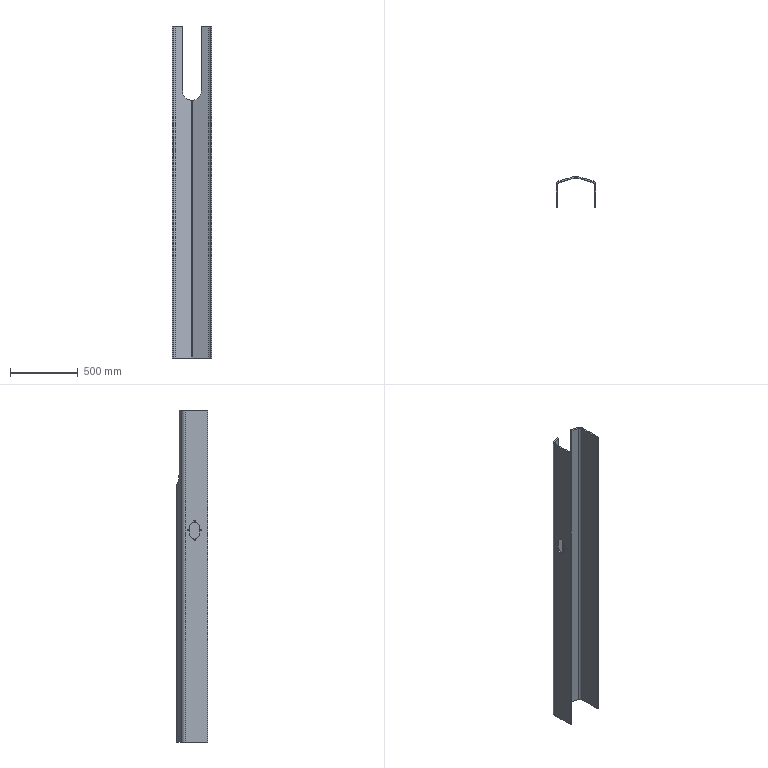Part | SolidWorks | features ICE 2, Extrusion 1, HoleWzd 1 | 1 solid | 36 faces | box 295 x 232 x 2455 mm | volume 15250128 mm3 | cylinder 19 | plane 17 | commonest cylinder face diameters 8.5 x8 40 x3 60 x3 80 x3 140 x2
STEP:
#1=CARTESIAN_POINT('',(-137.5,147.,1560.75));
#2=VERTEX_POINT('',#1);
#3=CARTESIAN_POINT('',(-137.5,147.,1569.25));
#4=VERTEX_POINT('',#3);
#5=CARTESIAN_POINT('',(-137.5,147.,1565.));
#6=DIRECTION('',(-1.,0.,0.));
#7=DIRECTION('',(0.,0.,1.));
#8=AXIS2_PLACEMENT_3D('',#5,#6,#7);
#9=CIRCLE('',#8,4.25);
#10=EDGE_CURVE('',#2,#4,#9,.T.);
#11=ORIENTED_EDGE('',*,*,#10,.F.);
#12=CARTESIAN_POINT('',(-147.5,147.,1560.75));
#13=VERTEX_POINT('',#12);
#14=CARTESIAN_POINT('',(-147.5,147.,1560.75));
#15=DIRECTION('',(-1.,0.,0.));
#16=VECTOR('',#15,1000.);
#17=LINE('',#14,#16);
#18=EDGE_CURVE('',#2,#13,#17,.T.);
#19=ORIENTED_EDGE('',*,*,#18,.T.);
#20=CARTESIAN_POINT('',(-147.5,147.,1569.25));
#21=VERTEX_POINT('',#20);
#22=CARTESIAN_POINT('',(-147.5,147.,1565.));
#23=DIRECTION('',(-1.,0.,0.));
#24=DIRECTION('',(0.,0.,1.));
#25=AXIS2_PLACEMENT_3D('',#22,#23,#24);
#26=CIRCLE('',#25,4.25);
#27=EDGE_CURVE('',#13,#21,#26,.T.);
#28=ORIENTED_EDGE('',*,*,#27,.T.);
#29=CARTESIAN_POINT('',(-147.5,147.,1569.25));
#30=DIRECTION('',(-1.,0.,0.));
#31=VECTOR('',#30,1000.);
#32=LINE('',#29,#31);
#33=EDGE_CURVE('',#4,#21,#32,.T.);
#34=ORIENTED_EDGE('',*,*,#33,.F.);
#35=EDGE_LOOP('',(#11,#19,#28,#34));
#36=FACE_OUTER_BOUND('',#35,.T.);
#37=CARTESIAN_POINT('',(-147.5,147.,1565.));
#38=DIRECTION('',(-1.,0.,0.));
#39=DIRECTION('',(0.,0.,1.));
#40=AXIS2_PLACEMENT_3D('',#37,#38,#39);
#41=CYLINDRICAL_SURFACE('',#40,4.25);
#42=ADVANCED_FACE('',(#36),#41,.F.);
#43=CARTESIAN_POINT('',(-137.5,47.,1560.75));
#44=VERTEX_POINT('',#43);
#45=CARTESIAN_POINT('',(-137.5,47.,1569.25));
#46=VERTEX_POINT('',#45);
#47=CARTESIAN_POINT('',(-137.5,47.,1565.));
#48=DIRECTION('',(-1.,0.,0.));
#49=DIRECTION('',(0.,0.,1.));
#50=AXIS2_PLACEMENT_3D('',#47,#48,#49);
#51=CIRCLE('',#50,4.25);
#52=EDGE_CURVE('',#44,#46,#51,.T.);
#53=ORIENTED_EDGE('',*,*,#52,.F.);
#54=CARTESIAN_POINT('',(-147.5,47.,1560.75));
#55=VERTEX_POINT('',#54);
#56=CARTESIAN_POINT('',(-147.5,47.,1560.75));
#57=DIRECTION('',(-1.,0.,0.));
#58=VECTOR('',#57,1000.);
#59=LINE('',#56,#58);
#60=EDGE_CURVE('',#44,#55,#59,.T.);
#61=ORIENTED_EDGE('',*,*,#60,.T.);
#62=CARTESIAN_POINT('',(-147.5,47.,1569.25));
#63=VERTEX_POINT('',#62);
#64=CARTESIAN_POINT('',(-147.5,47.,1565.));
#65=DIRECTION('',(-1.,0.,0.));
#66=DIRECTION('',(0.,0.,1.));
#67=AXIS2_PLACEMENT_3D('',#64,#65,#66);
#68=CIRCLE('',#67,4.25);
#69=EDGE_CURVE('',#55,#63,#68,.T.);
#70=ORIENTED_EDGE('',*,*,#69,.T.);
#71=CARTESIAN_POINT('',(-147.5,47.,1569.25));
#72=DIRECTION('',(-1.,0.,0.));
#73=VECTOR('',#72,1000.);
#74=LINE('',#71,#73);
#75=EDGE_CURVE('',#46,#63,#74,.T.);
#76=ORIENTED_EDGE('',*,*,#75,.F.);
#77=EDGE_LOOP('',(#53,#61,#70,#76));
#78=FACE_OUTER_BOUND('',#77,.T.);
#79=CARTESIAN_POINT('',(-147.5,47.,1565.));
#80=DIRECTION('',(-1.,0.,0.));
#81=DIRECTION('',(0.,0.,1.));
#82=AXIS2_PLACEMENT_3D('',#79,#80,#81);
#83=CYLINDRICAL_SURFACE('',#82,4.25);
#84=ADVANCED_FACE('',(#78),#83,.F.);
#85=CARTESIAN_POINT('',(-137.5,97.,1490.75));
#86=VERTEX_POINT('',#85);
#87=CARTESIAN_POINT('',(-137.5,97.,1499.25));
#88=VERTEX_POINT('',#87);
#89=CARTESIAN_POINT('',(-137.5,97.,1495.));
#90=DIRECTION('',(-1.,0.,0.));
#91=DIRECTION('',(0.,0.,1.));
#92=AXIS2_PLACEMENT_3D('',#89,#90,#91);
#93=CIRCLE('',#92,4.25);
#94=EDGE_CURVE('',#86,#88,#93,.T.);
#95=ORIENTED_EDGE('',*,*,#94,.F.);
#96=CARTESIAN_POINT('',(-147.5,97.,1490.75));
#97=VERTEX_POINT('',#96);
#98=CARTESIAN_POINT('',(-147.5,97.,1490.75));
#99=DIRECTION('',(-1.,0.,0.));
#100=VECTOR('',#99,1000.);
#101=LINE('',#98,#100);
#102=EDGE_CURVE('',#86,#97,#101,.T.);
#103=ORIENTED_EDGE('',*,*,#102,.T.);
#104=CARTESIAN_POINT('',(-147.5,97.,1499.25));
#105=VERTEX_POINT('',#104);
#106=CARTESIAN_POINT('',(-147.5,97.,1495.));
#107=DIRECTION('',(-1.,0.,0.));
#108=DIRECTION('',(0.,0.,1.));
#109=AXIS2_PLACEMENT_3D('',#106,#107,#108);
#110=CIRCLE('',#109,4.25);
#111=EDGE_CURVE('',#97,#105,#110,.T.);
#112=ORIENTED_EDGE('',*,*,#111,.T.);
#113=CARTESIAN_POINT('',(-147.5,97.,1499.25));
#114=DIRECTION('',(-1.,0.,0.));
#115=VECTOR('',#114,1000.);
#116=LINE('',#113,#115);
#117=EDGE_CURVE('',#88,#105,#116,.T.);
#118=ORIENTED_EDGE('',*,*,#117,.F.);
#119=EDGE_LOOP('',(#95,#103,#112,#118));
#120=FACE_OUTER_BOUND('',#119,.T.);
#121=CARTESIAN_POINT('',(-147.5,97.,1495.));
#122=DIRECTION('',(-1.,0.,0.));
#123=DIRECTION('',(0.,0.,1.));
#124=AXIS2_PLACEMENT_3D('',#121,#122,#123);
#125=CYLINDRICAL_SURFACE('',#124,4.25);
#126=ADVANCED_FACE('',(#120),#125,.F.);
#127=CARTESIAN_POINT('',(-137.5,97.,1630.75));
#128=VERTEX_POINT('',#127);
#129=CARTESIAN_POINT('',(-137.5,97.,1639.25));
#130=VERTEX_POINT('',#129);
#131=CARTESIAN_POINT('',(-137.5,97.,1635.));
#132=DIRECTION('',(-1.,0.,0.));
#133=DIRECTION('',(0.,0.,1.));
#134=AXIS2_PLACEMENT_3D('',#131,#132,#133);
#135=CIRCLE('',#134,4.25);
#136=EDGE_CURVE('',#128,#130,#135,.T.);
#137=ORIENTED_EDGE('',*,*,#136,.F.);
#138=CARTESIAN_POINT('',(-147.5,97.,1630.75));
#139=VERTEX_POINT('',#138);
#140=CARTESIAN_POINT('',(-147.5,97.,1630.75));
#141=DIRECTION('',(-1.,0.,0.));
#142=VECTOR('',#141,1000.);
#143=LINE('',#140,#142);
#144=EDGE_CURVE('',#128,#139,#143,.T.);
#145=ORIENTED_EDGE('',*,*,#144,.T.);
#146=CARTESIAN_POINT('',(-147.5,97.,1639.25));
#147=VERTEX_POINT('',#146);
#148=CARTESIAN_POINT('',(-147.5,97.,1635.));
#149=DIRECTION('',(-1.,0.,0.));
#150=DIRECTION('',(0.,0.,1.));
#151=AXIS2_PLACEMENT_3D('',#148,#149,#150);
#152=CIRCLE('',#151,4.25);
#153=EDGE_CURVE('',#139,#147,#152,.T.);
#154=ORIENTED_EDGE('',*,*,#153,.T.);
#155=CARTESIAN_POINT('',(-147.5,97.,1639.25));
#156=DIRECTION('',(-1.,0.,0.));
#157=VECTOR('',#156,1000.);
#158=LINE('',#155,#157);
#159=EDGE_CURVE('',#130,#147,#158,.T.);
#160=ORIENTED_EDGE('',*,*,#159,.F.);
#161=EDGE_LOOP('',(#137,#145,#154,#160));
#162=FACE_OUTER_BOUND('',#161,.T.);
#163=CARTESIAN_POINT('',(-147.5,97.,1635.));
#164=DIRECTION('',(-1.,0.,0.));
#165=DIRECTION('',(0.,0.,1.));
#166=AXIS2_PLACEMENT_3D('',#163,#164,#165);
#167=CYLINDRICAL_SURFACE('',#166,4.25);
#168=ADVANCED_FACE('',(#162),#167,.F.);
#169=CARTESIAN_POINT('',(-137.5,97.,1625.));
#170=VERTEX_POINT('',#169);
#171=CARTESIAN_POINT('',(-137.5,137.,1585.));
#172=VERTEX_POINT('',#171);
#173=CARTESIAN_POINT('',(-137.5,97.,1585.));
#174=DIRECTION('',(-1.,0.,0.));
#175=DIRECTION('',(0.,0.,1.));
#176=AXIS2_PLACEMENT_3D('',#173,#174,#175);
#177=CIRCLE('',#176,40.);
#178=EDGE_CURVE('',#170,#172,#177,.T.);
#179=ORIENTED_EDGE('',*,*,#178,.F.);
#180=CARTESIAN_POINT('',(-147.5,97.,1625.));
#181=VERTEX_POINT('',#180);
#182=CARTESIAN_POINT('',(-137.5,97.,1625.));
#183=DIRECTION('',(-1.,0.,0.));
#184=VECTOR('',#183,1000.);
#185=LINE('',#182,#184);
#186=EDGE_CURVE('',#170,#181,#185,.T.);
#187=ORIENTED_EDGE('',*,*,#186,.T.);
#188=CARTESIAN_POINT('',(-147.5,137.,1585.));
#189=VERTEX_POINT('',#188);
#190=CARTESIAN_POINT('',(-147.5,97.,1585.));
#191=DIRECTION('',(-1.,0.,0.));
#192=DIRECTION('',(0.,0.,1.));
#193=AXIS2_PLACEMENT_3D('',#190,#191,#192);
#194=CIRCLE('',#193,40.);
#195=EDGE_CURVE('',#181,#189,#194,.T.);
#196=ORIENTED_EDGE('',*,*,#195,.T.);
#197=CARTESIAN_POINT('',(-137.5,137.,1585.));
#198=DIRECTION('',(-1.,0.,0.));
#199=VECTOR('',#198,1000.);
#200=LINE('',#197,#199);
#201=EDGE_CURVE('',#172,#189,#200,.T.);
#202=ORIENTED_EDGE('',*,*,#201,.F.);
#203=EDGE_LOOP('',(#179,#187,#196,#202));
#204=FACE_OUTER_BOUND('',#203,.T.);
#205=CARTESIAN_POINT('',(-137.5,97.,1585.));
#206=DIRECTION('',(-1.,0.,0.));
#207=DIRECTION('',(0.,0.,1.));
#208=AXIS2_PLACEMENT_3D('',#205,#206,#207);
#209=CYLINDRICAL_SURFACE('',#208,40.);
#210=ADVANCED_FACE('',(#204),#209,.F.);
#211=CARTESIAN_POINT('',(8.771,230.689,1905.552));
#212=VERTEX_POINT('',#211);
#213=CARTESIAN_POINT('',(0.,232.,1905.));
#214=VERTEX_POINT('',#213);
#215=CARTESIAN_POINT('',(8.771,230.689,1905.552));
#216=CARTESIAN_POINT('',(7.345,231.125,1905.372));
#217=CARTESIAN_POINT('',(5.901,231.451,1905.234));
#218=CARTESIAN_POINT('',(2.978,231.888,1905.048));
#219=CARTESIAN_POINT('',(1.498,232.,1905.));
#220=CARTESIAN_POINT('',(0.,232.,1905.));
#221=B_SPLINE_CURVE_WITH_KNOTS('',3,(#215,#216,#217,#218,#219,#220),.UNSPECIFIED.,.F.,.F.,(4,2,4),(0.,0.004443,0.008885),.UNSPECIFIED.);
#222=EDGE_CURVE('',#212,#214,#221,.T.);
#223=ORIENTED_EDGE('',*,*,#222,.T.);
#224=CARTESIAN_POINT('',(0.,222.,1905.));
#225=VERTEX_POINT('',#224);
#226=CARTESIAN_POINT('',(0.,232.,1905.));
#227=DIRECTION('',(0.,-1.,0.));
#228=VECTOR('',#227,1000.);
#229=LINE('',#226,#228);
#230=EDGE_CURVE('',#214,#225,#229,.T.);
#231=ORIENTED_EDGE('',*,*,#230,.T.);
#232=CARTESIAN_POINT('',(5.847,221.126,1905.245));
#233=VERTEX_POINT('',#232);
#234=CARTESIAN_POINT('',(0.,222.,1905.));
#235=CARTESIAN_POINT('',(0.4958,222.,1905.));
#236=CARTESIAN_POINT('',(0.9948,221.981,1905.005));
#237=CARTESIAN_POINT('',(1.983,221.908,1905.026));
#238=CARTESIAN_POINT('',(2.473,221.853,1905.042));
#239=CARTESIAN_POINT('',(3.936,221.634,1905.104));
#240=CARTESIAN_POINT('',(4.898,221.416,1905.165));
#241=CARTESIAN_POINT('',(5.847,221.126,1905.245));
#242=B_SPLINE_CURVE_WITH_KNOTS('',3,(#234,#235,#236,#237,#238,#239,#240,#241),.UNSPECIFIED.,.F.,.F.,(4,2,2,4),(0.005917,0.00739,0.008863,0.01181),.UNSPECIFIED.);
#243=EDGE_CURVE('',#225,#233,#242,.T.);
#244=ORIENTED_EDGE('',*,*,#243,.T.);
#245=CARTESIAN_POINT('',(70.,201.513,1975.));
#246=VERTEX_POINT('',#245);
#247=CARTESIAN_POINT('',(5.847,221.126,1905.245));
#248=CARTESIAN_POINT('',(44.049,209.447,1908.447));
#249=CARTESIAN_POINT('',(70.,201.513,1936.664));
#250=CARTESIAN_POINT('',(70.,201.513,1975.));
#251=(BOUNDED_CURVE()B_SPLINE_CURVE(3,(#247,#248,#249,#250),.UNSPECIFIED.,.F.,.T.)B_SPLINE_CURVE_WITH_KNOTS((4,4),(4.796,6.283),.UNSPECIFIED.)CURVE()GEOMETRIC_REPRESENTATION_ITEM()RATIONAL_B_SPLINE_CURVE((1.,0.824,0.824,1.))REPRESENTATION_ITEM(''));
#252=EDGE_CURVE('',#233,#246,#251,.T.);
#253=ORIENTED_EDGE('',*,*,#252,.T.);
#254=CARTESIAN_POINT('',(70.,211.97,1975.));
#255=VERTEX_POINT('',#254);
#256=CARTESIAN_POINT('',(70.,232.,1975.));
#257=DIRECTION('',(0.,-1.,0.));
#258=VECTOR('',#257,1000.);
#259=LINE('',#256,#258);
#260=EDGE_CURVE('',#255,#246,#259,.T.);
#261=ORIENTED_EDGE('',*,*,#260,.F.);
#262=CARTESIAN_POINT('',(70.,211.97,1975.));
#263=CARTESIAN_POINT('',(70.,211.97,1937.969));
#264=CARTESIAN_POINT('',(45.51,219.457,1910.192));
#265=CARTESIAN_POINT('',(8.771,230.689,1905.552));
#266=(BOUNDED_CURVE()B_SPLINE_CURVE(3,(#262,#263,#264,#265),.UNSPECIFIED.,.F.,.T.)B_SPLINE_CURVE_WITH_KNOTS((4,4),(0.,1.445),.UNSPECIFIED.)CURVE()GEOMETRIC_REPRESENTATION_ITEM()RATIONAL_B_SPLINE_CURVE((1.,0.8334,0.8334,1.))REPRESENTATION_ITEM(''));
#267=EDGE_CURVE('',#255,#212,#266,.T.);
#268=ORIENTED_EDGE('',*,*,#267,.T.);
#269=EDGE_LOOP('',(#223,#231,#244,#253,#261,#268));
#270=FACE_OUTER_BOUND('',#269,.T.);
#271=CARTESIAN_POINT('',(0.,232.,1975.));
#272=DIRECTION('',(0.,-1.,0.));
#273=DIRECTION('',(0.,0.,-1.));
#274=AXIS2_PLACEMENT_3D('',#271,#272,#273);
#275=CYLINDRICAL_SURFACE('',#274,70.);
#276=ADVANCED_FACE('',(#270),#275,.F.);
#277=CARTESIAN_POINT('',(-70.,201.513,1975.));
#278=VERTEX_POINT('',#277);
#279=CARTESIAN_POINT('',(-5.847,221.126,1905.245));
#280=VERTEX_POINT('',#279);
#281=CARTESIAN_POINT('',(-70.,201.513,1975.));
#282=CARTESIAN_POINT('',(-70.,201.513,1936.664));
#283=CARTESIAN_POINT('',(-44.049,209.447,1908.447));
#284=CARTESIAN_POINT('',(-5.847,221.126,1905.245));
#285=(BOUNDED_CURVE()B_SPLINE_CURVE(3,(#281,#282,#283,#284),.UNSPECIFIED.,.F.,.T.)B_SPLINE_CURVE_WITH_KNOTS((4,4),(0.,1.487),.UNSPECIFIED.)CURVE()GEOMETRIC_REPRESENTATION_ITEM()RATIONAL_B_SPLINE_CURVE((1.,0.824,0.824,1.))REPRESENTATION_ITEM(''));
#286=EDGE_CURVE('',#278,#280,#285,.T.);
#287=ORIENTED_EDGE('',*,*,#286,.F.);
#288=CARTESIAN_POINT('',(-70.,201.513,2455.));
#289=VERTEX_POINT('',#288);
#290=CARTESIAN_POINT('',(-70.,201.513,2455.));
#291=DIRECTION('',(0.,0.,-1.));
#292=VECTOR('',#291,1000.);
#293=LINE('',#290,#292);
#294=EDGE_CURVE('',#289,#278,#293,.T.);
#295=ORIENTED_EDGE('',*,*,#294,.F.);
#296=CARTESIAN_POINT('',(-123.347,185.203,2455.));
#297=VERTEX_POINT('',#296);
#298=CARTESIAN_POINT('',(-123.347,185.203,2455.));
#299=DIRECTION('',(0.9563,0.2924,0.));
#300=VECTOR('',#299,1000.);
#301=LINE('',#298,#300);
#302=EDGE_CURVE('',#297,#289,#301,.T.);
#303=ORIENTED_EDGE('',*,*,#302,.F.);
#304=CARTESIAN_POINT('',(-123.347,185.203,0.));
#305=VERTEX_POINT('',#304);
#306=CARTESIAN_POINT('',(-123.347,185.203,2455.));
#307=DIRECTION('',(0.,0.,-1.));
#308=VECTOR('',#307,1000.);
#309=LINE('',#306,#308);
#310=EDGE_CURVE('',#297,#305,#309,.T.);
#311=ORIENTED_EDGE('',*,*,#310,.T.);
#312=CARTESIAN_POINT('',(-5.847,221.126,0.));
#313=VERTEX_POINT('',#312);
#314=CARTESIAN_POINT('',(-123.347,185.203,0.));
#315=DIRECTION('',(0.9563,0.2924,0.));
#316=VECTOR('',#315,1000.);
#317=LINE('',#314,#316);
#318=EDGE_CURVE('',#305,#313,#317,.T.);
#319=ORIENTED_EDGE('',*,*,#318,.T.);
#320=CARTESIAN_POINT('',(-5.847,221.126,2455.));
#321=DIRECTION('',(0.,0.,-1.));
#322=VECTOR('',#321,1000.);
#323=LINE('',#320,#322);
#324=EDGE_CURVE('',#280,#313,#323,.T.);
#325=ORIENTED_EDGE('',*,*,#324,.F.);
#326=EDGE_LOOP('',(#287,#295,#303,#311,#319,#325));
#327=FACE_OUTER_BOUND('',#326,.T.);
#328=CARTESIAN_POINT('',(-123.347,185.203,2455.));
#329=DIRECTION('',(-0.2924,0.9563,0.));
#330=DIRECTION('',(-0.9563,-0.2924,0.));
#331=AXIS2_PLACEMENT_3D('',#328,#329,#330);
#332=PLANE('',#331);
#333=ADVANCED_FACE('',(#327),#332,.F.);
#334=CARTESIAN_POINT('',(-5.847,221.126,1905.245));
#335=CARTESIAN_POINT('',(-4.894,221.418,1905.165));
#336=CARTESIAN_POINT('',(-3.93,221.635,1905.104));
#337=CARTESIAN_POINT('',(-1.981,221.926,1905.021));
#338=CARTESIAN_POINT('',(-0.9957,222.,1905.));
#339=CARTESIAN_POINT('',(0.,222.,1905.));
#340=B_SPLINE_CURVE_WITH_KNOTS('',3,(#334,#335,#336,#337,#338,#339),.UNSPECIFIED.,.F.,.F.,(4,2,4),(0.,0.002958,0.005917),.UNSPECIFIED.);
#341=EDGE_CURVE('',#280,#225,#340,.T.);
#342=ORIENTED_EDGE('',*,*,#341,.F.);
#343=ORIENTED_EDGE('',*,*,#324,.T.);
#344=CARTESIAN_POINT('',(5.847,221.126,0.));
#345=VERTEX_POINT('',#344);
#346=CARTESIAN_POINT('',(0.,202.,0.));
#347=DIRECTION('',(0.,0.,-1.));
#348=DIRECTION('',(1.,0.,0.));
#349=AXIS2_PLACEMENT_3D('',#346,#347,#348);
#350=CIRCLE('',#349,20.);
#351=EDGE_CURVE('',#313,#345,#350,.T.);
#352=ORIENTED_EDGE('',*,*,#351,.T.);
#353=CARTESIAN_POINT('',(5.847,221.126,2455.));
#354=DIRECTION('',(0.,0.,-1.));
#355=VECTOR('',#354,1000.);
#356=LINE('',#353,#355);
#357=EDGE_CURVE('',#233,#345,#356,.T.);
#358=ORIENTED_EDGE('',*,*,#357,.F.);
#359=ORIENTED_EDGE('',*,*,#243,.F.);
#360=EDGE_LOOP('',(#342,#343,#352,#358,#359));
#361=FACE_OUTER_BOUND('',#360,.T.);
#362=CARTESIAN_POINT('',(0.,202.,2455.));
#363=DIRECTION('',(0.,0.,-1.));
#364=DIRECTION('',(-1.,0.,0.));
#365=AXIS2_PLACEMENT_3D('',#362,#363,#364);
#366=CYLINDRICAL_SURFACE('',#365,20.);
#367=ADVANCED_FACE('',(#361),#366,.F.);
#368=ORIENTED_EDGE('',*,*,#252,.F.);
#369=ORIENTED_EDGE('',*,*,#357,.T.);
#370=CARTESIAN_POINT('',(123.347,185.203,0.));
#371=VERTEX_POINT('',#370);
#372=CARTESIAN_POINT('',(123.347,185.203,0.));
#373=DIRECTION('',(0.9563,-0.2924,0.));
#374=VECTOR('',#373,1000.);
#375=LINE('',#372,#374);
#376=EDGE_CURVE('',#345,#371,#375,.T.);
#377=ORIENTED_EDGE('',*,*,#376,.T.);
#378=CARTESIAN_POINT('',(123.347,185.203,2455.));
#379=VERTEX_POINT('',#378);
#380=CARTESIAN_POINT('',(123.347,185.203,2455.));
#381=DIRECTION('',(0.,0.,-1.));
#382=VECTOR('',#381,1000.);
#383=LINE('',#380,#382);
#384=EDGE_CURVE('',#379,#371,#383,.T.);
#385=ORIENTED_EDGE('',*,*,#384,.F.);
#386=CARTESIAN_POINT('',(70.,201.513,2455.));
#387=VERTEX_POINT('',#386);
#388=CARTESIAN_POINT('',(123.347,185.203,2455.));
#389=DIRECTION('',(0.9563,-0.2924,0.));
#390=VECTOR('',#389,1000.);
#391=LINE('',#388,#390);
#392=EDGE_CURVE('',#387,#379,#391,.T.);
#393=ORIENTED_EDGE('',*,*,#392,.F.);
#394=CARTESIAN_POINT('',(70.,201.513,2455.));
#395=DIRECTION('',(0.,0.,1.));
#396=VECTOR('',#395,1000.);
#397=LINE('',#394,#396);
#398=EDGE_CURVE('',#246,#387,#397,.T.);
#399=ORIENTED_EDGE('',*,*,#398,.F.);
#400=EDGE_LOOP('',(#368,#369,#377,#385,#393,#399));
#401=FACE_OUTER_BOUND('',#400,.T.);
#402=CARTESIAN_POINT('',(123.347,185.203,2455.));
#403=DIRECTION('',(0.2924,0.9563,0.));
#404=DIRECTION('',(-0.9563,0.2924,0.));
#405=AXIS2_PLACEMENT_3D('',#402,#403,#404);
#406=PLANE('',#405);
#407=ADVANCED_FACE('',(#401),#406,.F.);
#408=ORIENTED_EDGE('',*,*,#267,.F.);
#409=CARTESIAN_POINT('',(70.,211.97,2455.));
#410=VERTEX_POINT('',#409);
#411=CARTESIAN_POINT('',(70.,211.97,2455.));
#412=DIRECTION('',(0.,0.,-1.));
#413=VECTOR('',#412,1000.);
#414=LINE('',#411,#413);
#415=EDGE_CURVE('',#410,#255,#414,.T.);
#416=ORIENTED_EDGE('',*,*,#415,.F.);
#417=CARTESIAN_POINT('',(126.271,194.766,2455.));
#418=VERTEX_POINT('',#417);
#419=CARTESIAN_POINT('',(126.271,194.766,2455.));
#420=DIRECTION('',(-0.9563,0.2924,0.));
#421=VECTOR('',#420,1000.);
#422=LINE('',#419,#421);
#423=EDGE_CURVE('',#418,#410,#422,.T.);
#424=ORIENTED_EDGE('',*,*,#423,.F.);
#425=CARTESIAN_POINT('',(126.271,194.766,0.));
#426=VERTEX_POINT('',#425);
#427=CARTESIAN_POINT('',(126.271,194.766,2455.));
#428=DIRECTION('',(0.,0.,-1.));
#429=VECTOR('',#428,1000.);
#430=LINE('',#427,#429);
#431=EDGE_CURVE('',#418,#426,#430,.T.);
#432=ORIENTED_EDGE('',*,*,#431,.T.);
#433=CARTESIAN_POINT('',(8.771,230.689,0.));
#434=VERTEX_POINT('',#433);
#435=CARTESIAN_POINT('',(126.271,194.766,0.));
#436=DIRECTION('',(-0.9563,0.2924,0.));
#437=VECTOR('',#436,1000.);
#438=LINE('',#435,#437);
#439=EDGE_CURVE('',#426,#434,#438,.T.);
#440=ORIENTED_EDGE('',*,*,#439,.T.);
#441=CARTESIAN_POINT('',(8.771,230.689,2455.));
#442=DIRECTION('',(0.,0.,-1.));
#443=VECTOR('',#442,1000.);
#444=LINE('',#441,#443);
#445=EDGE_CURVE('',#212,#434,#444,.T.);
#446=ORIENTED_EDGE('',*,*,#445,.F.);
#447=EDGE_LOOP('',(#408,#416,#424,#432,#440,#446));
#448=FACE_OUTER_BOUND('',#447,.T.);
#449=CARTESIAN_POINT('',(126.271,194.766,2455.));
#450=DIRECTION('',(-0.2924,-0.9563,0.));
#451=DIRECTION('',(0.9563,-0.2924,0.));
#452=AXIS2_PLACEMENT_3D('',#449,#450,#451);
#453=PLANE('',#452);
#454=ADVANCED_FACE('',(#448),#453,.F.);
#455=ORIENTED_EDGE('',*,*,#222,.F.);
#456=ORIENTED_EDGE('',*,*,#445,.T.);
#457=CARTESIAN_POINT('',(-8.771,230.689,0.));
#458=VERTEX_POINT('',#457);
#459=CARTESIAN_POINT('',(0.,202.,0.));
#460=DIRECTION('',(0.,0.,1.));
#461=DIRECTION('',(1.,0.,0.));
#462=AXIS2_PLACEMENT_3D('',#459,#460,#461);
#463=CIRCLE('',#462,30.);
#464=EDGE_CURVE('',#434,#458,#463,.T.);
#465=ORIENTED_EDGE('',*,*,#464,.T.);
#466=CARTESIAN_POINT('',(-8.771,230.689,1905.552));
#467=VERTEX_POINT('',#466);
#468=CARTESIAN_POINT('',(-8.771,230.689,2455.));
#469=DIRECTION('',(0.,0.,-1.));
#470=VECTOR('',#469,1000.);
#471=LINE('',#468,#470);
#472=EDGE_CURVE('',#467,#458,#471,.T.);
#473=ORIENTED_EDGE('',*,*,#472,.F.);
#474=CARTESIAN_POINT('',(0.,232.,1905.));
#475=CARTESIAN_POINT('',(-0.747,232.,1905.));
#476=CARTESIAN_POINT('',(-1.496,231.972,1905.012));
#477=CARTESIAN_POINT('',(-2.978,231.861,1905.059));
#478=CARTESIAN_POINT('',(-3.714,231.778,1905.095));
#479=CARTESIAN_POINT('',(-5.907,231.45,1905.234));
#480=CARTESIAN_POINT('',(-7.349,231.124,1905.372));
#481=CARTESIAN_POINT('',(-8.771,230.689,1905.552));
#482=B_SPLINE_CURVE_WITH_KNOTS('',3,(#474,#475,#476,#477,#478,#479,#480,#481),.UNSPECIFIED.,.F.,.F.,(4,2,2,4),(0.008885,0.0111,0.01332,0.01775),.UNSPECIFIED.);
#483=EDGE_CURVE('',#214,#467,#482,.T.);
#484=ORIENTED_EDGE('',*,*,#483,.F.);
#485=EDGE_LOOP('',(#455,#456,#465,#473,#484));
#486=FACE_OUTER_BOUND('',#485,.T.);
#487=CARTESIAN_POINT('',(0.,202.,2455.));
#488=DIRECTION('',(0.,0.,-1.));
#489=DIRECTION('',(-1.,0.,0.));
#490=AXIS2_PLACEMENT_3D('',#487,#488,#489);
#491=CYLINDRICAL_SURFACE('',#490,30.);
#492=ADVANCED_FACE('',(#486),#491,.T.);
#493=CARTESIAN_POINT('',(-70.,211.97,1975.));
#494=VERTEX_POINT('',#493);
#495=CARTESIAN_POINT('',(-8.771,230.689,1905.552));
#496=CARTESIAN_POINT('',(-45.51,219.457,1910.192));
#497=CARTESIAN_POINT('',(-70.,211.97,1937.969));
#498=CARTESIAN_POINT('',(-70.,211.97,1975.));
#499=(BOUNDED_CURVE()B_SPLINE_CURVE(3,(#495,#496,#497,#498),.UNSPECIFIED.,.F.,.F.)B_SPLINE_CURVE_WITH_KNOTS((4,4),(4.838,6.283),.UNSPECIFIED.)CURVE()GEOMETRIC_REPRESENTATION_ITEM()RATIONAL_B_SPLINE_CURVE((1.,0.8334,0.8334,1.))REPRESENTATION_ITEM(''));
#500=EDGE_CURVE('',#467,#494,#499,.T.);
#501=ORIENTED_EDGE('',*,*,#500,.F.);
#502=ORIENTED_EDGE('',*,*,#472,.T.);
#503=CARTESIAN_POINT('',(-126.271,194.766,0.));
#504=VERTEX_POINT('',#503);
#505=CARTESIAN_POINT('',(-126.271,194.766,0.));
#506=DIRECTION('',(-0.9563,-0.2924,0.));
#507=VECTOR('',#506,1000.);
#508=LINE('',#505,#507);
#509=EDGE_CURVE('',#458,#504,#508,.T.);
#510=ORIENTED_EDGE('',*,*,#509,.T.);
#511=CARTESIAN_POINT('',(-126.271,194.766,2455.));
#512=VERTEX_POINT('',#511);
#513=CARTESIAN_POINT('',(-126.271,194.766,2455.));
#514=DIRECTION('',(0.,0.,-1.));
#515=VECTOR('',#514,1000.);
#516=LINE('',#513,#515);
#517=EDGE_CURVE('',#512,#504,#516,.T.);
#518=ORIENTED_EDGE('',*,*,#517,.F.);
#519=CARTESIAN_POINT('',(-70.,211.97,2455.));
#520=VERTEX_POINT('',#519);
#521=CARTESIAN_POINT('',(-126.271,194.766,2455.));
#522=DIRECTION('',(-0.9563,-0.2924,0.));
#523=VECTOR('',#522,1000.);
#524=LINE('',#521,#523);
#525=EDGE_CURVE('',#520,#512,#524,.T.);
#526=ORIENTED_EDGE('',*,*,#525,.F.);
#527=CARTESIAN_POINT('',(-70.,211.97,2455.));
#528=DIRECTION('',(0.,0.,1.));
#529=VECTOR('',#528,1000.);
#530=LINE('',#527,#529);
#531=EDGE_CURVE('',#494,#520,#530,.T.);
#532=ORIENTED_EDGE('',*,*,#531,.F.);
#533=EDGE_LOOP('',(#501,#502,#510,#518,#526,#532));
#534=FACE_OUTER_BOUND('',#533,.T.);
#535=CARTESIAN_POINT('',(-126.271,194.766,2455.));
#536=DIRECTION('',(0.2924,-0.9563,0.));
#537=DIRECTION('',(0.9563,0.2924,0.));
#538=AXIS2_PLACEMENT_3D('',#535,#536,#537);
#539=PLANE('',#538);
#540=ADVANCED_FACE('',(#534),#539,.F.);
#541=CARTESIAN_POINT('',(-70.,166.077,2455.));
#542=DIRECTION('',(0.,-1.,0.));
#543=VECTOR('',#542,1000.);
#544=LINE('',#541,#543);
#545=EDGE_CURVE('',#520,#289,#544,.T.);
#546=ORIENTED_EDGE('',*,*,#545,.F.);
#547=ORIENTED_EDGE('',*,*,#525,.T.);
#548=CARTESIAN_POINT('',(-147.5,166.077,2455.));
#549=VERTEX_POINT('',#548);
#550=CARTESIAN_POINT('',(-117.5,166.077,2455.));
#551=DIRECTION('',(0.,0.,1.));
#552=DIRECTION('',(-1.,0.,0.));
#553=AXIS2_PLACEMENT_3D('',#550,#551,#552);
#554=CIRCLE('',#553,30.);
#555=EDGE_CURVE('',#512,#549,#554,.T.);
#556=ORIENTED_EDGE('',*,*,#555,.T.);
#557=CARTESIAN_POINT('',(-147.5,0.,2455.));
#558=VERTEX_POINT('',#557);
#559=CARTESIAN_POINT('',(-147.5,0.,2455.));
#560=DIRECTION('',(0.,-1.,0.));
#561=VECTOR('',#560,1000.);
#562=LINE('',#559,#561);
#563=EDGE_CURVE('',#549,#558,#562,.T.);
#564=ORIENTED_EDGE('',*,*,#563,.T.);
#565=CARTESIAN_POINT('',(-137.5,0.,2455.));
#566=VERTEX_POINT('',#565);
#567=CARTESIAN_POINT('',(-147.5,0.,2455.));
#568=DIRECTION('',(1.,0.,0.));
#569=VECTOR('',#568,1000.);
#570=LINE('',#567,#569);
#571=EDGE_CURVE('',#558,#566,#570,.T.);
#572=ORIENTED_EDGE('',*,*,#571,.T.);
#573=CARTESIAN_POINT('',(-137.5,166.077,2455.));
#574=VERTEX_POINT('',#573);
#575=CARTESIAN_POINT('',(-137.5,0.,2455.));
#576=DIRECTION('',(0.,1.,0.));
#577=VECTOR('',#576,1000.);
#578=LINE('',#575,#577);
#579=EDGE_CURVE('',#566,#574,#578,.T.);
#580=ORIENTED_EDGE('',*,*,#579,.T.);
#581=CARTESIAN_POINT('',(-117.5,166.077,2455.));
#582=DIRECTION('',(0.,0.,-1.));
#583=DIRECTION('',(-1.,0.,0.));
#584=AXIS2_PLACEMENT_3D('',#581,#582,#583);
#585=CIRCLE('',#584,20.);
#586=EDGE_CURVE('',#574,#297,#585,.T.);
#587=ORIENTED_EDGE('',*,*,#586,.T.);
#588=ORIENTED_EDGE('',*,*,#302,.T.);
#589=EDGE_LOOP('',(#546,#547,#556,#564,#572,#580,#587,#588));
#590=FACE_OUTER_BOUND('',#589,.T.);
#591=CARTESIAN_POINT('',(-117.5,166.077,2455.));
#592=DIRECTION('',(0.,0.,-1.));
#593=DIRECTION('',(-1.,0.,0.));
#594=AXIS2_PLACEMENT_3D('',#591,#592,#593);
#595=PLANE('',#594);
#596=ADVANCED_FACE('',(#590),#595,.F.);
#597=CARTESIAN_POINT('',(70.,166.077,2455.));
#598=DIRECTION('',(0.,1.,0.));
#599=VECTOR('',#598,1000.);
#600=LINE('',#597,#599);
#601=EDGE_CURVE('',#387,#410,#600,.T.);
#602=ORIENTED_EDGE('',*,*,#601,.F.);
#603=ORIENTED_EDGE('',*,*,#392,.T.);
#604=CARTESIAN_POINT('',(137.5,166.077,2455.));
#605=VERTEX_POINT('',#604);
#606=CARTESIAN_POINT('',(117.5,166.077,2455.));
#607=DIRECTION('',(0.,0.,-1.));
#608=DIRECTION('',(1.,0.,0.));
#609=AXIS2_PLACEMENT_3D('',#606,#607,#608);
#610=CIRCLE('',#609,20.);
#611=EDGE_CURVE('',#379,#605,#610,.T.);
#612=ORIENTED_EDGE('',*,*,#611,.T.);
#613=CARTESIAN_POINT('',(137.5,0.,2455.));
#614=VERTEX_POINT('',#613);
#615=CARTESIAN_POINT('',(137.5,166.077,2455.));
#616=DIRECTION('',(0.,-1.,0.));
#617=VECTOR('',#616,1000.);
#618=LINE('',#615,#617);
#619=EDGE_CURVE('',#605,#614,#618,.T.);
#620=ORIENTED_EDGE('',*,*,#619,.T.);
#621=CARTESIAN_POINT('',(147.5,0.,2455.));
#622=VERTEX_POINT('',#621);
#623=CARTESIAN_POINT('',(137.5,0.,2455.));
#624=DIRECTION('',(1.,0.,0.));
#625=VECTOR('',#624,1000.);
#626=LINE('',#623,#625);
#627=EDGE_CURVE('',#614,#622,#626,.T.);
#628=ORIENTED_EDGE('',*,*,#627,.T.);
#629=CARTESIAN_POINT('',(147.5,166.077,2455.));
#630=VERTEX_POINT('',#629);
#631=CARTESIAN_POINT('',(147.5,166.077,2455.));
#632=DIRECTION('',(0.,1.,0.));
#633=VECTOR('',#632,1000.);
#634=LINE('',#631,#633);
#635=EDGE_CURVE('',#622,#630,#634,.T.);
#636=ORIENTED_EDGE('',*,*,#635,.T.);
#637=CARTESIAN_POINT('',(117.5,166.077,2455.));
#638=DIRECTION('',(0.,0.,1.));
#639=DIRECTION('',(1.,0.,0.));
#640=AXIS2_PLACEMENT_3D('',#637,#638,#639);
#641=CIRCLE('',#640,30.);
#642=EDGE_CURVE('',#630,#418,#641,.T.);
#643=ORIENTED_EDGE('',*,*,#642,.T.);
#644=ORIENTED_EDGE('',*,*,#423,.T.);
#645=EDGE_LOOP('',(#602,#603,#612,#620,#628,#636,#643,#644));
#646=FACE_OUTER_BOUND('',#645,.T.);
#647=CARTESIAN_POINT('',(-117.5,166.077,2455.));
#648=DIRECTION('',(0.,0.,-1.));
#649=DIRECTION('',(-1.,0.,0.));
#650=AXIS2_PLACEMENT_3D('',#647,#648,#649);
#651=PLANE('',#650);
#652=ADVANCED_FACE('',(#646),#651,.F.);
#653=CARTESIAN_POINT('',(-147.5,0.,0.));
#654=VERTEX_POINT('',#653);
#655=CARTESIAN_POINT('',(-137.5,0.,0.));
#656=VERTEX_POINT('',#655);
#657=CARTESIAN_POINT('',(-147.5,0.,0.));
#658=DIRECTION('',(1.,0.,0.));
#659=VECTOR('',#658,1000.);
#660=LINE('',#657,#659);
#661=EDGE_CURVE('',#654,#656,#660,.T.);
#662=ORIENTED_EDGE('',*,*,#661,.T.);
#663=CARTESIAN_POINT('',(-137.5,0.,2455.));
#664=DIRECTION('',(0.,0.,-1.));
#665=VECTOR('',#664,1000.);
#666=LINE('',#663,#665);
#667=EDGE_CURVE('',#566,#656,#666,.T.);
#668=ORIENTED_EDGE('',*,*,#667,.F.);
#669=ORIENTED_EDGE('',*,*,#571,.F.);
#670=CARTESIAN_POINT('',(-147.5,0.,2455.));
#671=DIRECTION('',(0.,0.,-1.));
#672=VECTOR('',#671,1000.);
#673=LINE('',#670,#672);
#674=EDGE_CURVE('',#558,#654,#673,.T.);
#675=ORIENTED_EDGE('',*,*,#674,.T.);
#676=EDGE_LOOP('',(#662,#668,#669,#675));
#677=FACE_OUTER_BOUND('',#676,.T.);
#678=CARTESIAN_POINT('',(-147.5,0.,2455.));
#679=DIRECTION('',(0.,1.,0.));
#680=DIRECTION('',(0.,0.,1.));
#681=AXIS2_PLACEMENT_3D('',#678,#679,#680);
#682=PLANE('',#681);
#683=ADVANCED_FACE('',(#677),#682,.F.);
#684=CARTESIAN_POINT('',(-137.5,147.,1565.));
#685=DIRECTION('',(-1.,0.,0.));
#686=DIRECTION('',(0.,0.,1.));
#687=AXIS2_PLACEMENT_3D('',#684,#685,#686);
#688=CIRCLE('',#687,4.25);
#689=EDGE_CURVE('',#4,#2,#688,.T.);
#690=ORIENTED_EDGE('',*,*,#689,.T.);
#691=ORIENTED_EDGE('',*,*,#10,.T.);
#692=EDGE_LOOP('',(#690,#691));
#693=FACE_BOUND('',#692,.T.);
#694=CARTESIAN_POINT('',(-137.5,47.,1565.));
#695=DIRECTION('',(-1.,0.,0.));
#696=DIRECTION('',(0.,0.,1.));
#697=AXIS2_PLACEMENT_3D('',#694,#695,#696);
#698=CIRCLE('',#697,4.25);
#699=EDGE_CURVE('',#46,#44,#698,.T.);
#700=ORIENTED_EDGE('',*,*,#699,.T.);
#701=ORIENTED_EDGE('',*,*,#52,.T.);
#702=EDGE_LOOP('',(#700,#701));
#703=FACE_BOUND('',#702,.T.);
#704=CARTESIAN_POINT('',(-137.5,97.,1495.));
#705=DIRECTION('',(-1.,0.,0.));
#706=DIRECTION('',(0.,0.,1.));
#707=AXIS2_PLACEMENT_3D('',#704,#705,#706);
#708=CIRCLE('',#707,4.25);
#709=EDGE_CURVE('',#88,#86,#708,.T.);
#710=ORIENTED_EDGE('',*,*,#709,.T.);
#711=ORIENTED_EDGE('',*,*,#94,.T.);
#712=EDGE_LOOP('',(#710,#711));
#713=FACE_BOUND('',#712,.T.);
#714=CARTESIAN_POINT('',(-137.5,97.,1635.));
#715=DIRECTION('',(-1.,0.,0.));
#716=DIRECTION('',(0.,0.,1.));
#717=AXIS2_PLACEMENT_3D('',#714,#715,#716);
#718=CIRCLE('',#717,4.25);
#719=EDGE_CURVE('',#130,#128,#718,.T.);
#720=ORIENTED_EDGE('',*,*,#719,.T.);
#721=ORIENTED_EDGE('',*,*,#136,.T.);
#722=EDGE_LOOP('',(#720,#721));
#723=FACE_BOUND('',#722,.T.);
#724=CARTESIAN_POINT('',(-137.5,57.,1545.));
#725=VERTEX_POINT('',#724);
#726=CARTESIAN_POINT('',(-137.5,57.,1585.));
#727=VERTEX_POINT('',#726);
#728=CARTESIAN_POINT('',(-137.5,57.,1545.));
#729=DIRECTION('',(0.,0.,1.));
#730=VECTOR('',#729,1000.);
#731=LINE('',#728,#730);
#732=EDGE_CURVE('',#725,#727,#731,.T.);
#733=ORIENTED_EDGE('',*,*,#732,.T.);
#734=CARTESIAN_POINT('',(-137.5,97.,1585.));
#735=DIRECTION('',(-1.,0.,0.));
#736=DIRECTION('',(0.,0.,1.));
#737=AXIS2_PLACEMENT_3D('',#734,#735,#736);
#738=CIRCLE('',#737,40.);
#739=EDGE_CURVE('',#727,#170,#738,.T.);
#740=ORIENTED_EDGE('',*,*,#739,.T.);
#741=ORIENTED_EDGE('',*,*,#178,.T.);
#742=CARTESIAN_POINT('',(-137.5,137.,1545.));
#743=VERTEX_POINT('',#742);
#744=CARTESIAN_POINT('',(-137.5,137.,1545.));
#745=DIRECTION('',(0.,0.,-1.));
#746=VECTOR('',#745,1000.);
#747=LINE('',#744,#746);
#748=EDGE_CURVE('',#172,#743,#747,.T.);
#749=ORIENTED_EDGE('',*,*,#748,.T.);
#750=CARTESIAN_POINT('',(-137.5,97.,1545.));
#751=DIRECTION('',(-1.,0.,0.));
#752=DIRECTION('',(0.,0.,1.));
#753=AXIS2_PLACEMENT_3D('',#750,#751,#752);
#754=CIRCLE('',#753,40.);
#755=EDGE_CURVE('',#743,#725,#754,.T.);
#756=ORIENTED_EDGE('',*,*,#755,.T.);
#757=EDGE_LOOP('',(#733,#740,#741,#749,#756));
#758=FACE_BOUND('',#757,.T.);
#759=CARTESIAN_POINT('',(-137.5,166.077,0.));
#760=VERTEX_POINT('',#759);
#761=CARTESIAN_POINT('',(-137.5,0.,0.));
#762=DIRECTION('',(0.,1.,0.));
#763=VECTOR('',#762,1000.);
#764=LINE('',#761,#763);
#765=EDGE_CURVE('',#656,#760,#764,.T.);
#766=ORIENTED_EDGE('',*,*,#765,.T.);
#767=CARTESIAN_POINT('',(-137.5,166.077,2455.));
#768=DIRECTION('',(0.,0.,-1.));
#769=VECTOR('',#768,1000.);
#770=LINE('',#767,#769);
#771=EDGE_CURVE('',#574,#760,#770,.T.);
#772=ORIENTED_EDGE('',*,*,#771,.F.);
#773=ORIENTED_EDGE('',*,*,#579,.F.);
#774=ORIENTED_EDGE('',*,*,#667,.T.);
#775=EDGE_LOOP('',(#766,#772,#773,#774));
#776=FACE_OUTER_BOUND('',#775,.T.);
#777=CARTESIAN_POINT('',(-137.5,0.,2455.));
#778=DIRECTION('',(-1.,0.,0.));
#779=DIRECTION('',(0.,0.,1.));
#780=AXIS2_PLACEMENT_3D('',#777,#778,#779);
#781=PLANE('',#780);
#782=ADVANCED_FACE('',(#693,#703,#713,#723,#758,#776),#781,.F.);
#783=CARTESIAN_POINT('',(-117.5,166.077,0.));
#784=DIRECTION('',(0.,0.,-1.));
#785=DIRECTION('',(-1.,0.,0.));
#786=AXIS2_PLACEMENT_3D('',#783,#784,#785);
#787=CIRCLE('',#786,20.);
#788=EDGE_CURVE('',#760,#305,#787,.T.);
#789=ORIENTED_EDGE('',*,*,#788,.T.);
#790=ORIENTED_EDGE('',*,*,#310,.F.);
#791=ORIENTED_EDGE('',*,*,#586,.F.);
#792=ORIENTED_EDGE('',*,*,#771,.T.);
#793=EDGE_LOOP('',(#789,#790,#791,#792));
#794=FACE_OUTER_BOUND('',#793,.T.);
#795=CARTESIAN_POINT('',(-117.5,166.077,2455.));
#796=DIRECTION('',(0.,0.,-1.));
#797=DIRECTION('',(-1.,0.,0.));
#798=AXIS2_PLACEMENT_3D('',#795,#796,#797);
#799=CYLINDRICAL_SURFACE('',#798,20.);
#800=ADVANCED_FACE('',(#794),#799,.F.);
#801=CARTESIAN_POINT('',(137.5,166.077,0.));
#802=VERTEX_POINT('',#801);
#803=CARTESIAN_POINT('',(117.5,166.077,0.));
#804=DIRECTION('',(0.,0.,-1.));
#805=DIRECTION('',(1.,0.,0.));
#806=AXIS2_PLACEMENT_3D('',#803,#804,#805);
#807=CIRCLE('',#806,20.);
#808=EDGE_CURVE('',#371,#802,#807,.T.);
#809=ORIENTED_EDGE('',*,*,#808,.T.);
#810=CARTESIAN_POINT('',(137.5,166.077,2455.));
#811=DIRECTION('',(0.,0.,-1.));
#812=VECTOR('',#811,1000.);
#813=LINE('',#810,#812);
#814=EDGE_CURVE('',#605,#802,#813,.T.);
#815=ORIENTED_EDGE('',*,*,#814,.F.);
#816=ORIENTED_EDGE('',*,*,#611,.F.);
#817=ORIENTED_EDGE('',*,*,#384,.T.);
#818=EDGE_LOOP('',(#809,#815,#816,#817));
#819=FACE_OUTER_BOUND('',#818,.T.);
#820=CARTESIAN_POINT('',(117.5,166.077,2455.));
#821=DIRECTION('',(0.,0.,-1.));
#822=DIRECTION('',(-1.,0.,0.));
#823=AXIS2_PLACEMENT_3D('',#820,#821,#822);
#824=CYLINDRICAL_SURFACE('',#823,20.);
#825=ADVANCED_FACE('',(#819),#824,.F.);
#826=CARTESIAN_POINT('',(137.5,0.,0.));
#827=VERTEX_POINT('',#826);
#828=CARTESIAN_POINT('',(137.5,166.077,0.));
#829=DIRECTION('',(0.,-1.,0.));
#830=VECTOR('',#829,1000.);
#831=LINE('',#828,#830);
#832=EDGE_CURVE('',#802,#827,#831,.T.);
#833=ORIENTED_EDGE('',*,*,#832,.T.);
#834=CARTESIAN_POINT('',(137.5,0.,2455.));
#835=DIRECTION('',(0.,0.,-1.));
#836=VECTOR('',#835,1000.);
#837=LINE('',#834,#836);
#838=EDGE_CURVE('',#614,#827,#837,.T.);
#839=ORIENTED_EDGE('',*,*,#838,.F.);
#840=ORIENTED_EDGE('',*,*,#619,.F.);
#841=ORIENTED_EDGE('',*,*,#814,.T.);
#842=EDGE_LOOP('',(#833,#839,#840,#841));
#843=FACE_OUTER_BOUND('',#842,.T.);
#844=CARTESIAN_POINT('',(137.5,166.077,2455.));
#845=DIRECTION('',(1.,0.,0.));
#846=DIRECTION('',(0.,0.,-1.));
#847=AXIS2_PLACEMENT_3D('',#844,#845,#846);
#848=PLANE('',#847);
#849=ADVANCED_FACE('',(#843),#848,.F.);
#850=CARTESIAN_POINT('',(147.5,0.,0.));
#851=VERTEX_POINT('',#850);
#852=CARTESIAN_POINT('',(137.5,0.,0.));
#853=DIRECTION('',(1.,0.,0.));
#854=VECTOR('',#853,1000.);
#855=LINE('',#852,#854);
#856=EDGE_CURVE('',#827,#851,#855,.T.);
#857=ORIENTED_EDGE('',*,*,#856,.T.);
#858=CARTESIAN_POINT('',(147.5,0.,2455.));
#859=DIRECTION('',(0.,0.,-1.));
#860=VECTOR('',#859,1000.);
#861=LINE('',#858,#860);
#862=EDGE_CURVE('',#622,#851,#861,.T.);
#863=ORIENTED_EDGE('',*,*,#862,.F.);
#864=ORIENTED_EDGE('',*,*,#627,.F.);
#865=ORIENTED_EDGE('',*,*,#838,.T.);
#866=EDGE_LOOP('',(#857,#863,#864,#865));
#867=FACE_OUTER_BOUND('',#866,.T.);
#868=CARTESIAN_POINT('',(137.5,0.,2455.));
#869=DIRECTION('',(0.,1.,0.));
#870=DIRECTION('',(-1.,0.,0.));
#871=AXIS2_PLACEMENT_3D('',#868,#869,#870);
#872=PLANE('',#871);
#873=ADVANCED_FACE('',(#867),#872,.F.);
#874=CARTESIAN_POINT('',(147.5,166.077,0.));
#875=VERTEX_POINT('',#874);
#876=CARTESIAN_POINT('',(147.5,166.077,0.));
#877=DIRECTION('',(0.,1.,0.));
#878=VECTOR('',#877,1000.);
#879=LINE('',#876,#878);
#880=EDGE_CURVE('',#851,#875,#879,.T.);
#881=ORIENTED_EDGE('',*,*,#880,.T.);
#882=CARTESIAN_POINT('',(147.5,166.077,2455.));
#883=DIRECTION('',(0.,0.,-1.));
#884=VECTOR('',#883,1000.);
#885=LINE('',#882,#884);
#886=EDGE_CURVE('',#630,#875,#885,.T.);
#887=ORIENTED_EDGE('',*,*,#886,.F.);
#888=ORIENTED_EDGE('',*,*,#635,.F.);
#889=ORIENTED_EDGE('',*,*,#862,.T.);
#890=EDGE_LOOP('',(#881,#887,#888,#889));
#891=FACE_OUTER_BOUND('',#890,.T.);
#892=CARTESIAN_POINT('',(147.5,166.077,2455.));
#893=DIRECTION('',(-1.,0.,0.));
#894=DIRECTION('',(0.,-1.,0.));
#895=AXIS2_PLACEMENT_3D('',#892,#893,#894);
#896=PLANE('',#895);
#897=ADVANCED_FACE('',(#891),#896,.F.);
#898=CARTESIAN_POINT('',(117.5,166.077,0.));
#899=DIRECTION('',(0.,0.,1.));
#900=DIRECTION('',(1.,0.,0.));
#901=AXIS2_PLACEMENT_3D('',#898,#899,#900);
#902=CIRCLE('',#901,30.);
#903=EDGE_CURVE('',#875,#426,#902,.T.);
#904=ORIENTED_EDGE('',*,*,#903,.T.);
#905=ORIENTED_EDGE('',*,*,#431,.F.);
#906=ORIENTED_EDGE('',*,*,#642,.F.);
#907=ORIENTED_EDGE('',*,*,#886,.T.);
#908=EDGE_LOOP('',(#904,#905,#906,#907));
#909=FACE_OUTER_BOUND('',#908,.T.);
#910=CARTESIAN_POINT('',(117.5,166.077,2455.));
#911=DIRECTION('',(0.,0.,-1.));
#912=DIRECTION('',(-1.,0.,0.));
#913=AXIS2_PLACEMENT_3D('',#910,#911,#912);
#914=CYLINDRICAL_SURFACE('',#913,30.);
#915=ADVANCED_FACE('',(#909),#914,.T.);
#916=CARTESIAN_POINT('',(-147.5,166.077,0.));
#917=VERTEX_POINT('',#916);
#918=CARTESIAN_POINT('',(-117.5,166.077,0.));
#919=DIRECTION('',(0.,0.,1.));
#920=DIRECTION('',(-1.,0.,0.));
#921=AXIS2_PLACEMENT_3D('',#918,#919,#920);
#922=CIRCLE('',#921,30.);
#923=EDGE_CURVE('',#504,#917,#922,.T.);
#924=ORIENTED_EDGE('',*,*,#923,.T.);
#925=CARTESIAN_POINT('',(-147.5,166.077,2455.));
#926=DIRECTION('',(0.,0.,-1.));
#927=VECTOR('',#926,1000.);
#928=LINE('',#925,#927);
#929=EDGE_CURVE('',#549,#917,#928,.T.);
#930=ORIENTED_EDGE('',*,*,#929,.F.);
#931=ORIENTED_EDGE('',*,*,#555,.F.);
#932=ORIENTED_EDGE('',*,*,#517,.T.);
#933=EDGE_LOOP('',(#924,#930,#931,#932));
#934=FACE_OUTER_BOUND('',#933,.T.);
#935=CARTESIAN_POINT('',(-117.5,166.077,2455.));
#936=DIRECTION('',(0.,0.,-1.));
#937=DIRECTION('',(-1.,0.,0.));
#938=AXIS2_PLACEMENT_3D('',#935,#936,#937);
#939=CYLINDRICAL_SURFACE('',#938,30.);
#940=ADVANCED_FACE('',(#934),#939,.T.);
#941=CARTESIAN_POINT('',(-147.5,147.,1565.));
#942=DIRECTION('',(-1.,0.,0.));
#943=DIRECTION('',(0.,0.,1.));
#944=AXIS2_PLACEMENT_3D('',#941,#942,#943);
#945=CIRCLE('',#944,4.25);
#946=EDGE_CURVE('',#21,#13,#945,.T.);
#947=ORIENTED_EDGE('',*,*,#946,.F.);
#948=ORIENTED_EDGE('',*,*,#27,.F.);
#949=EDGE_LOOP('',(#947,#948));
#950=FACE_BOUND('',#949,.T.);
#951=CARTESIAN_POINT('',(-147.5,47.,1565.));
#952=DIRECTION('',(-1.,0.,0.));
#953=DIRECTION('',(0.,0.,1.));
#954=AXIS2_PLACEMENT_3D('',#951,#952,#953);
#955=CIRCLE('',#954,4.25);
#956=EDGE_CURVE('',#63,#55,#955,.T.);
#957=ORIENTED_EDGE('',*,*,#956,.F.);
#958=ORIENTED_EDGE('',*,*,#69,.F.);
#959=EDGE_LOOP('',(#957,#958));
#960=FACE_BOUND('',#959,.T.);
#961=CARTESIAN_POINT('',(-147.5,97.,1495.));
#962=DIRECTION('',(-1.,0.,0.));
#963=DIRECTION('',(0.,0.,1.));
#964=AXIS2_PLACEMENT_3D('',#961,#962,#963);
#965=CIRCLE('',#964,4.25);
#966=EDGE_CURVE('',#105,#97,#965,.T.);
#967=ORIENTED_EDGE('',*,*,#966,.F.);
#968=ORIENTED_EDGE('',*,*,#111,.F.);
#969=EDGE_LOOP('',(#967,#968));
#970=FACE_BOUND('',#969,.T.);
#971=CARTESIAN_POINT('',(-147.5,97.,1635.));
#972=DIRECTION('',(-1.,0.,0.));
#973=DIRECTION('',(0.,0.,1.));
#974=AXIS2_PLACEMENT_3D('',#971,#972,#973);
#975=CIRCLE('',#974,4.25);
#976=EDGE_CURVE('',#147,#139,#975,.T.);
#977=ORIENTED_EDGE('',*,*,#976,.F.);
#978=ORIENTED_EDGE('',*,*,#153,.F.);
#979=EDGE_LOOP('',(#977,#978));
#980=FACE_BOUND('',#979,.T.);
#981=CARTESIAN_POINT('',(-147.5,137.,1545.));
#982=VERTEX_POINT('',#981);
#983=CARTESIAN_POINT('',(-147.5,137.,1545.));
#984=DIRECTION('',(0.,0.,-1.));
#985=VECTOR('',#984,1000.);
#986=LINE('',#983,#985);
#987=EDGE_CURVE('',#189,#982,#986,.T.);
#988=ORIENTED_EDGE('',*,*,#987,.F.);
#989=ORIENTED_EDGE('',*,*,#195,.F.);
#990=CARTESIAN_POINT('',(-147.5,57.,1585.));
#991=VERTEX_POINT('',#990);
#992=CARTESIAN_POINT('',(-147.5,97.,1585.));
#993=DIRECTION('',(-1.,0.,0.));
#994=DIRECTION('',(0.,0.,1.));
#995=AXIS2_PLACEMENT_3D('',#992,#993,#994);
#996=CIRCLE('',#995,40.);
#997=EDGE_CURVE('',#991,#181,#996,.T.);
#998=ORIENTED_EDGE('',*,*,#997,.F.);
#999=CARTESIAN_POINT('',(-147.5,57.,1545.));
#1000=VERTEX_POINT('',#999);
#1001=CARTESIAN_POINT('',(-147.5,57.,1545.));
#1002=DIRECTION('',(0.,0.,1.));
#1003=VECTOR('',#1002,1000.);
#1004=LINE('',#1001,#1003);
#1005=EDGE_CURVE('',#1000,#991,#1004,.T.);
#1006=ORIENTED_EDGE('',*,*,#1005,.F.);
#1007=CARTESIAN_POINT('',(-147.5,97.,1545.));
#1008=DIRECTION('',(-1.,0.,0.));
#1009=DIRECTION('',(0.,0.,1.));
#1010=AXIS2_PLACEMENT_3D('',#1007,#1008,#1009);
#1011=CIRCLE('',#1010,40.);
#1012=EDGE_CURVE('',#982,#1000,#1011,.T.);
#1013=ORIENTED_EDGE('',*,*,#1012,.F.);
#1014=EDGE_LOOP('',(#988,#989,#998,#1006,#1013));
#1015=FACE_BOUND('',#1014,.T.);
#1016=CARTESIAN_POINT('',(-147.5,0.,0.));
#1017=DIRECTION('',(0.,-1.,0.));
#1018=VECTOR('',#1017,1000.);
#1019=LINE('',#1016,#1018);
#1020=EDGE_CURVE('',#917,#654,#1019,.T.);
#1021=ORIENTED_EDGE('',*,*,#1020,.T.);
#1022=ORIENTED_EDGE('',*,*,#674,.F.);
#1023=ORIENTED_EDGE('',*,*,#563,.F.);
#1024=ORIENTED_EDGE('',*,*,#929,.T.);
#1025=EDGE_LOOP('',(#1021,#1022,#1023,#1024));
#1026=FACE_OUTER_BOUND('',#1025,.T.);
#1027=CARTESIAN_POINT('',(-147.5,0.,2455.));
#1028=DIRECTION('',(1.,0.,0.));
#1029=DIRECTION('',(0.,0.,-1.));
#1030=AXIS2_PLACEMENT_3D('',#1027,#1028,#1029);
#1031=PLANE('',#1030);
#1032=ADVANCED_FACE('',(#950,#960,#970,#980,#1015,#1026),#1031,.F.);
#1033=ORIENTED_EDGE('',*,*,#661,.F.);
#1034=ORIENTED_EDGE('',*,*,#1020,.F.);
#1035=ORIENTED_EDGE('',*,*,#923,.F.);
#1036=ORIENTED_EDGE('',*,*,#509,.F.);
#1037=ORIENTED_EDGE('',*,*,#464,.F.);
#1038=ORIENTED_EDGE('',*,*,#439,.F.);
#1039=ORIENTED_EDGE('',*,*,#903,.F.);
#1040=ORIENTED_EDGE('',*,*,#880,.F.);
#1041=ORIENTED_EDGE('',*,*,#856,.F.);
#1042=ORIENTED_EDGE('',*,*,#832,.F.);
#1043=ORIENTED_EDGE('',*,*,#808,.F.);
#1044=ORIENTED_EDGE('',*,*,#376,.F.);
#1045=ORIENTED_EDGE('',*,*,#351,.F.);
#1046=ORIENTED_EDGE('',*,*,#318,.F.);
#1047=ORIENTED_EDGE('',*,*,#788,.F.);
#1048=ORIENTED_EDGE('',*,*,#765,.F.);
#1049=EDGE_LOOP('',(#1033,#1034,#1035,#1036,#1037,#1038,#1039,#1040,#1041,#1042,#1043,#1044,#1045,#1046,#1047,#1048));
#1050=FACE_OUTER_BOUND('',#1049,.T.);
#1051=CARTESIAN_POINT('',(-117.5,166.077,0.));
#1052=DIRECTION('',(0.,0.,-1.));
#1053=DIRECTION('',(-1.,0.,0.));
#1054=AXIS2_PLACEMENT_3D('',#1051,#1052,#1053);
#1055=PLANE('',#1054);
#1056=ADVANCED_FACE('',(#1050),#1055,.T.);
#1057=ORIENTED_EDGE('',*,*,#230,.F.);
#1058=ORIENTED_EDGE('',*,*,#483,.T.);
#1059=ORIENTED_EDGE('',*,*,#500,.T.);
#1060=CARTESIAN_POINT('',(-70.,232.,1975.));
#1061=DIRECTION('',(0.,-1.,0.));
#1062=VECTOR('',#1061,1000.);
#1063=LINE('',#1060,#1062);
#1064=EDGE_CURVE('',#494,#278,#1063,.T.);
#1065=ORIENTED_EDGE('',*,*,#1064,.T.);
#1066=ORIENTED_EDGE('',*,*,#286,.T.);
#1067=ORIENTED_EDGE('',*,*,#341,.T.);
#1068=EDGE_LOOP('',(#1057,#1058,#1059,#1065,#1066,#1067));
#1069=FACE_OUTER_BOUND('',#1068,.T.);
#1070=CARTESIAN_POINT('',(0.,232.,1975.));
#1071=DIRECTION('',(0.,-1.,0.));
#1072=DIRECTION('',(0.,0.,-1.));
#1073=AXIS2_PLACEMENT_3D('',#1070,#1071,#1072);
#1074=CYLINDRICAL_SURFACE('',#1073,70.);
#1075=ADVANCED_FACE('',(#1069),#1074,.F.);
#1076=ORIENTED_EDGE('',*,*,#294,.T.);
#1077=ORIENTED_EDGE('',*,*,#1064,.F.);
#1078=ORIENTED_EDGE('',*,*,#531,.T.);
#1079=ORIENTED_EDGE('',*,*,#545,.T.);
#1080=EDGE_LOOP('',(#1076,#1077,#1078,#1079));
#1081=FACE_OUTER_BOUND('',#1080,.T.);
#1082=CARTESIAN_POINT('',(-70.,232.,1975.));
#1083=DIRECTION('',(1.,0.,0.));
#1084=DIRECTION('',(0.,0.,-1.));
#1085=AXIS2_PLACEMENT_3D('',#1082,#1083,#1084);
#1086=PLANE('',#1085);
#1087=ADVANCED_FACE('',(#1081),#1086,.T.);
#1088=ORIENTED_EDGE('',*,*,#398,.T.);
#1089=ORIENTED_EDGE('',*,*,#601,.T.);
#1090=ORIENTED_EDGE('',*,*,#415,.T.);
#1091=ORIENTED_EDGE('',*,*,#260,.T.);
#1092=EDGE_LOOP('',(#1088,#1089,#1090,#1091));
#1093=FACE_OUTER_BOUND('',#1092,.T.);
#1094=CARTESIAN_POINT('',(70.,232.,1975.));
#1095=DIRECTION('',(-1.,0.,0.));
#1096=DIRECTION('',(0.,0.,1.));
#1097=AXIS2_PLACEMENT_3D('',#1094,#1095,#1096);
#1098=PLANE('',#1097);
#1099=ADVANCED_FACE('',(#1093),#1098,.T.);
#1100=ORIENTED_EDGE('',*,*,#186,.F.);
#1101=ORIENTED_EDGE('',*,*,#739,.F.);
#1102=CARTESIAN_POINT('',(-137.5,57.,1585.));
#1103=DIRECTION('',(-1.,0.,0.));
#1104=VECTOR('',#1103,1000.);
#1105=LINE('',#1102,#1104);
#1106=EDGE_CURVE('',#727,#991,#1105,.T.);
#1107=ORIENTED_EDGE('',*,*,#1106,.T.);
#1108=ORIENTED_EDGE('',*,*,#997,.T.);
#1109=EDGE_LOOP('',(#1100,#1101,#1107,#1108));
#1110=FACE_OUTER_BOUND('',#1109,.T.);
#1111=CARTESIAN_POINT('',(-137.5,97.,1585.));
#1112=DIRECTION('',(-1.,0.,0.));
#1113=DIRECTION('',(0.,0.,1.));
#1114=AXIS2_PLACEMENT_3D('',#1111,#1112,#1113);
#1115=CYLINDRICAL_SURFACE('',#1114,40.);
#1116=ADVANCED_FACE('',(#1110),#1115,.F.);
#1117=ORIENTED_EDGE('',*,*,#1005,.T.);
#1118=ORIENTED_EDGE('',*,*,#1106,.F.);
#1119=ORIENTED_EDGE('',*,*,#732,.F.);
#1120=CARTESIAN_POINT('',(-137.5,57.,1545.));
#1121=DIRECTION('',(-1.,0.,0.));
#1122=VECTOR('',#1121,1000.);
#1123=LINE('',#1120,#1122);
#1124=EDGE_CURVE('',#725,#1000,#1123,.T.);
#1125=ORIENTED_EDGE('',*,*,#1124,.T.);
#1126=EDGE_LOOP('',(#1117,#1118,#1119,#1125));
#1127=FACE_OUTER_BOUND('',#1126,.T.);
#1128=CARTESIAN_POINT('',(-137.5,57.,1545.));
#1129=DIRECTION('',(0.,-1.,0.));
#1130=DIRECTION('',(0.,0.,-1.));
#1131=AXIS2_PLACEMENT_3D('',#1128,#1129,#1130);
#1132=PLANE('',#1131);
#1133=ADVANCED_FACE('',(#1127),#1132,.F.);
#1134=ORIENTED_EDGE('',*,*,#1012,.T.);
#1135=ORIENTED_EDGE('',*,*,#1124,.F.);
#1136=ORIENTED_EDGE('',*,*,#755,.F.);
#1137=CARTESIAN_POINT('',(-137.5,137.,1545.));
#1138=DIRECTION('',(-1.,0.,0.));
#1139=VECTOR('',#1138,1000.);
#1140=LINE('',#1137,#1139);
#1141=EDGE_CURVE('',#743,#982,#1140,.T.);
#1142=ORIENTED_EDGE('',*,*,#1141,.T.);
#1143=EDGE_LOOP('',(#1134,#1135,#1136,#1142));
#1144=FACE_OUTER_BOUND('',#1143,.T.);
#1145=CARTESIAN_POINT('',(-137.5,97.,1545.));
#1146=DIRECTION('',(-1.,0.,0.));
#1147=DIRECTION('',(0.,0.,1.));
#1148=AXIS2_PLACEMENT_3D('',#1145,#1146,#1147);
#1149=CYLINDRICAL_SURFACE('',#1148,40.);
#1150=ADVANCED_FACE('',(#1144),#1149,.F.);
#1151=ORIENTED_EDGE('',*,*,#987,.T.);
#1152=ORIENTED_EDGE('',*,*,#1141,.F.);
#1153=ORIENTED_EDGE('',*,*,#748,.F.);
#1154=ORIENTED_EDGE('',*,*,#201,.T.);
#1155=EDGE_LOOP('',(#1151,#1152,#1153,#1154));
#1156=FACE_OUTER_BOUND('',#1155,.T.);
#1157=CARTESIAN_POINT('',(-137.5,137.,1545.));
#1158=DIRECTION('',(0.,1.,0.));
#1159=DIRECTION('',(0.,0.,1.));
#1160=AXIS2_PLACEMENT_3D('',#1157,#1158,#1159);
#1161=PLANE('',#1160);
#1162=ADVANCED_FACE('',(#1156),#1161,.F.);
#1163=ORIENTED_EDGE('',*,*,#144,.F.);
#1164=ORIENTED_EDGE('',*,*,#719,.F.);
#1165=ORIENTED_EDGE('',*,*,#159,.T.);
#1166=ORIENTED_EDGE('',*,*,#976,.T.);
#1167=EDGE_LOOP('',(#1163,#1164,#1165,#1166));
#1168=FACE_OUTER_BOUND('',#1167,.T.);
#1169=CARTESIAN_POINT('',(-147.5,97.,1635.));
#1170=DIRECTION('',(-1.,0.,0.));
#1171=DIRECTION('',(0.,0.,1.));
#1172=AXIS2_PLACEMENT_3D('',#1169,#1170,#1171);
#1173=CYLINDRICAL_SURFACE('',#1172,4.25);
#1174=ADVANCED_FACE('',(#1168),#1173,.F.);
#1175=ORIENTED_EDGE('',*,*,#102,.F.);
#1176=ORIENTED_EDGE('',*,*,#709,.F.);
#1177=ORIENTED_EDGE('',*,*,#117,.T.);
#1178=ORIENTED_EDGE('',*,*,#966,.T.);
#1179=EDGE_LOOP('',(#1175,#1176,#1177,#1178));
#1180=FACE_OUTER_BOUND('',#1179,.T.);
#1181=CARTESIAN_POINT('',(-147.5,97.,1495.));
#1182=DIRECTION('',(-1.,0.,0.));
#1183=DIRECTION('',(0.,0.,1.));
#1184=AXIS2_PLACEMENT_3D('',#1181,#1182,#1183);
#1185=CYLINDRICAL_SURFACE('',#1184,4.25);
#1186=ADVANCED_FACE('',(#1180),#1185,.F.);
#1187=ORIENTED_EDGE('',*,*,#60,.F.);
#1188=ORIENTED_EDGE('',*,*,#699,.F.);
#1189=ORIENTED_EDGE('',*,*,#75,.T.);
#1190=ORIENTED_EDGE('',*,*,#956,.T.);
#1191=EDGE_LOOP('',(#1187,#1188,#1189,#1190));
#1192=FACE_OUTER_BOUND('',#1191,.T.);
#1193=CARTESIAN_POINT('',(-147.5,47.,1565.));
#1194=DIRECTION('',(-1.,0.,0.));
#1195=DIRECTION('',(0.,0.,1.));
#1196=AXIS2_PLACEMENT_3D('',#1193,#1194,#1195);
#1197=CYLINDRICAL_SURFACE('',#1196,4.25);
#1198=ADVANCED_FACE('',(#1192),#1197,.F.);
#1199=ORIENTED_EDGE('',*,*,#18,.F.);
#1200=ORIENTED_EDGE('',*,*,#689,.F.);
#1201=ORIENTED_EDGE('',*,*,#33,.T.);
#1202=ORIENTED_EDGE('',*,*,#946,.T.);
#1203=EDGE_LOOP('',(#1199,#1200,#1201,#1202));
#1204=FACE_OUTER_BOUND('',#1203,.T.);
#1205=CARTESIAN_POINT('',(-147.5,147.,1565.));
#1206=DIRECTION('',(-1.,0.,0.));
#1207=DIRECTION('',(0.,0.,1.));
#1208=AXIS2_PLACEMENT_3D('',#1205,#1206,#1207);
#1209=CYLINDRICAL_SURFACE('',#1208,4.25);
#1210=ADVANCED_FACE('',(#1204),#1209,.F.);
#1211=CLOSED_SHELL('',(#42,#84,#126,#168,#210,#276,#333,#367,#407,#454,#492,#540,#596,#652,#683,#782,#800,#825,#849,#873,#897,#915,#940,#1032,#1056,#1075,#1087,#1099,#1116,#1133,#1150,#1162,#1174,#1186,#1198,#1210));
#1212=MANIFOLD_SOLID_BREP('',#1211);
#1213=CARTESIAN_POINT('',(0.,0.,0.));
#1214=DIRECTION('',(0.,0.,1.));
#1215=DIRECTION('',(1.,0.,0.));
#1216=AXIS2_PLACEMENT_3D('',#1213,#1214,#1215);
#1217=(LENGTH_UNIT()NAMED_UNIT(*)SI_UNIT(.MILLI.,.METRE.));
#1218=UNCERTAINTY_MEASURE_WITH_UNIT(LENGTH_MEASURE(0.00001),#1217,'','');
#1219=(NAMED_UNIT(*)PLANE_ANGLE_UNIT()SI_UNIT($,.RADIAN.));
#1220=(NAMED_UNIT(*)SI_UNIT($,.STERADIAN.)SOLID_ANGLE_UNIT());
#1221=(GEOMETRIC_REPRESENTATION_CONTEXT(3)GLOBAL_UNCERTAINTY_ASSIGNED_CONTEXT((#1218))GLOBAL_UNIT_ASSIGNED_CONTEXT((#1217,#1219,#1220))REPRESENTATION_CONTEXT('',''));
#1222=ADVANCED_BREP_SHAPE_REPRESENTATION('',(#1212,#1216),#1221);